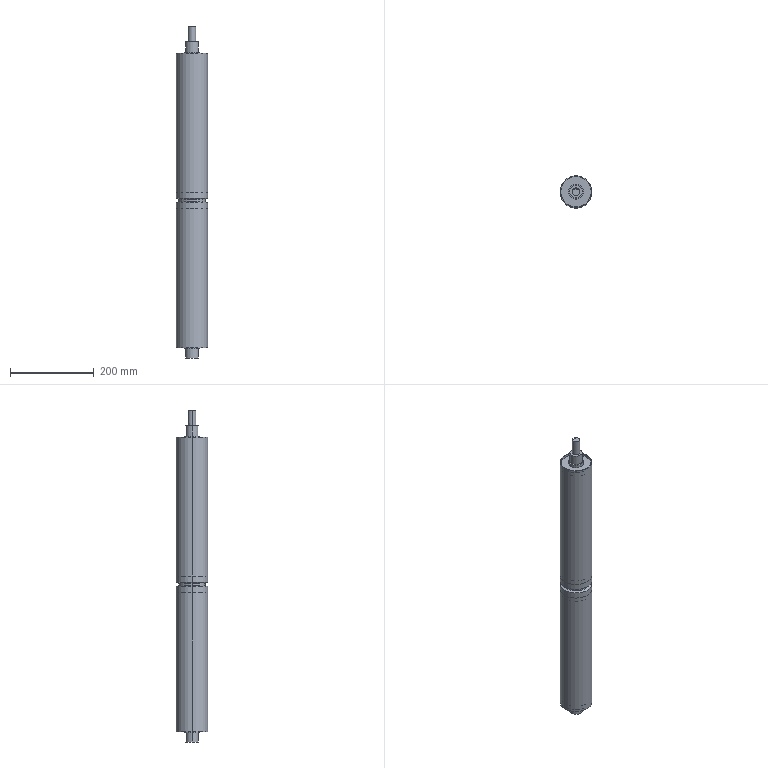Part | SolidWorks | features ICE 9, Extrusion 1, RevCut 1, Revolution 1 | 6 solids | 61 faces | box 76 x 76 x 795 mm | volume 1220082 mm3 | cylinder 37 | plane 20 | cone 4 | commonest cylinder face diameters 73 x12 35 x8 76 x8 30 x4 18 x2 64 x2